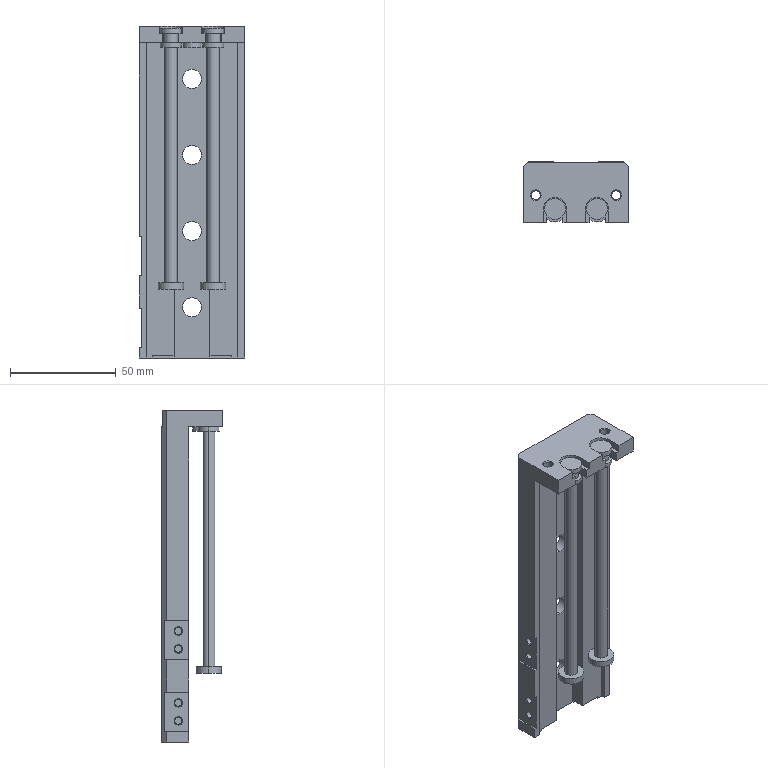Part | SolidWorks | features BaseBody 1 | 1 solid | 202 faces | box 50 x 29 x 157 mm | volume 83904 mm3 | plane 107 | cylinder 71 | cone 24 | commonest cylinder face diameters 3.242 x20 9 x8 10 x8 4 x5 4.134 x4 4.9 x4